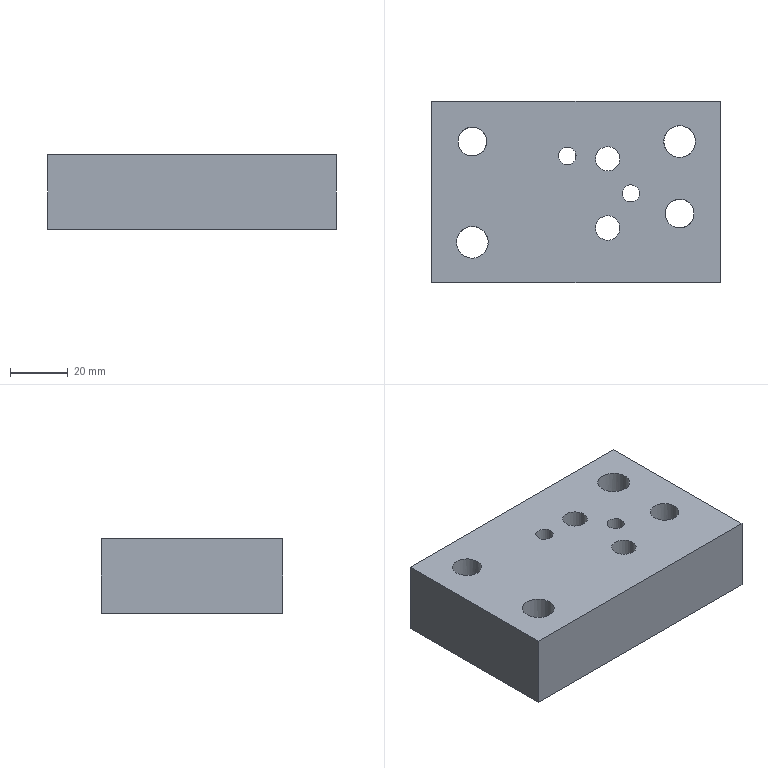Part | STEP file | 104_id42_x_t | 1 solid | 24 faces | box 100 x 63 x 26 mm | volume 145550 mm3 | cylinder 12 | plane 10 | cone 2 | commonest cylinder face diameters 6 x2 8.5 x2 10 x2 11 x2 12 x2 17 x2